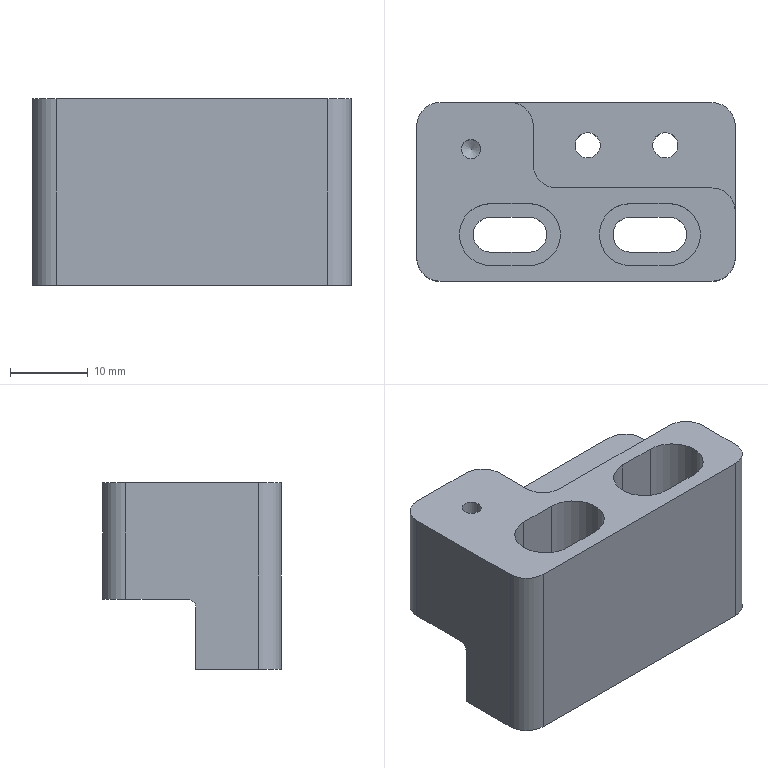Part | 1 solid | 41 faces | box 41 x 23 x 24 mm | volume 12874 mm3 | plane 21 | cylinder 19 | cone 1 | commonest cylinder face diameters 6 x7 4.5 x4 8 x4 3.242 x2 2 x1 2.459 x1
STEP:
#1=CARTESIAN_POINT('',(-14.729,5.5,-8.));
#2=VERTEX_POINT('',#1);
#3=CARTESIAN_POINT('',(-13.5,5.5,-8.));
#4=DIRECTION('',(0.,0.,1.));
#5=DIRECTION('',(-1.,0.,0.));
#6=AXIS2_PLACEMENT_3D('',#3,#4,#5);
#7=CIRCLE('',#6,1.23);
#8=EDGE_CURVE('',#2,#2,#7,.T.);
#9=ORIENTED_EDGE('',*,*,#8,.F.);
#10=EDGE_LOOP('',(#9));
#11=FACE_BOUND('',#10,.T.);
#12=CARTESIAN_POINT('',(-14.729,5.5,0.));
#13=VERTEX_POINT('',#12);
#14=CARTESIAN_POINT('',(-13.5,5.5,0.));
#15=DIRECTION('',(0.,0.,1.));
#16=DIRECTION('',(-1.,0.,0.));
#17=AXIS2_PLACEMENT_3D('',#14,#15,#16);
#18=CIRCLE('',#17,1.23);
#19=EDGE_CURVE('',#13,#13,#18,.T.);
#20=ORIENTED_EDGE('',*,*,#19,.T.);
#21=EDGE_LOOP('',(#20));
#22=FACE_BOUND('',#21,.T.);
#23=CARTESIAN_POINT('',(-13.5,5.5,0.));
#24=DIRECTION('',(0.,0.,-1.));
#25=DIRECTION('',(-1.,0.,0.));
#26=AXIS2_PLACEMENT_3D('',#23,#24,#25);
#27=CYLINDRICAL_SURFACE('',#26,1.23);
#28=ADVANCED_FACE('',(#11,#22),#27,.F.);
#29=CARTESIAN_POINT('',(-2.5,0.5,-7.5));
#30=VERTEX_POINT('',#29);
#31=CARTESIAN_POINT('',(17.5,0.5,-7.5));
#32=VERTEX_POINT('',#31);
#33=CARTESIAN_POINT('',(7.5,0.5,-7.5));
#34=DIRECTION('',(1.,0.,0.));
#35=VECTOR('',#34,1000.);
#36=LINE('',#33,#35);
#37=EDGE_CURVE('',#30,#32,#36,.T.);
#38=ORIENTED_EDGE('',*,*,#37,.F.);
#39=CARTESIAN_POINT('',(-2.5,0.5,0.));
#40=VERTEX_POINT('',#39);
#41=CARTESIAN_POINT('',(-2.5,0.5,-3.75));
#42=DIRECTION('',(0.,0.,-1.));
#43=VECTOR('',#42,1000.);
#44=LINE('',#41,#43);
#45=EDGE_CURVE('',#40,#30,#44,.T.);
#46=ORIENTED_EDGE('',*,*,#45,.F.);
#47=CARTESIAN_POINT('',(17.5,0.5,0.));
#48=VERTEX_POINT('',#47);
#49=CARTESIAN_POINT('',(7.5,0.5,0.));
#50=DIRECTION('',(1.,0.,0.));
#51=VECTOR('',#50,1000.);
#52=LINE('',#49,#51);
#53=EDGE_CURVE('',#40,#48,#52,.T.);
#54=ORIENTED_EDGE('',*,*,#53,.T.);
#55=CARTESIAN_POINT('',(17.5,0.5,-12.));
#56=DIRECTION('',(0.,0.,-1.));
#57=VECTOR('',#56,1000.);
#58=LINE('',#55,#57);
#59=EDGE_CURVE('',#48,#32,#58,.T.);
#60=ORIENTED_EDGE('',*,*,#59,.T.);
#61=EDGE_LOOP('',(#38,#46,#54,#60));
#62=FACE_BOUND('',#61,.T.);
#63=CARTESIAN_POINT('',(-5.5,0.5,0.));
#64=DIRECTION('',(0.,1.,0.));
#65=DIRECTION('',(1.,0.,0.));
#66=AXIS2_PLACEMENT_3D('',#63,#64,#65);
#67=PLANE('',#66);
#68=ADVANCED_FACE('',(#62),#67,.T.);
#69=CARTESIAN_POINT('',(-5.5,8.5,0.));
#70=VERTEX_POINT('',#69);
#71=CARTESIAN_POINT('',(-5.5,8.5,-7.5));
#72=VERTEX_POINT('',#71);
#73=CARTESIAN_POINT('',(-5.5,8.5,-7.5));
#74=DIRECTION('',(0.,0.,-1.));
#75=VECTOR('',#74,1000.);
#76=LINE('',#73,#75);
#77=EDGE_CURVE('',#70,#72,#76,.T.);
#78=ORIENTED_EDGE('',*,*,#77,.F.);
#79=CARTESIAN_POINT('',(-5.5,3.5,0.));
#80=VERTEX_POINT('',#79);
#81=CARTESIAN_POINT('',(-5.5,6.,0.));
#82=DIRECTION('',(0.,1.,0.));
#83=VECTOR('',#82,1000.);
#84=LINE('',#81,#83);
#85=EDGE_CURVE('',#80,#70,#84,.T.);
#86=ORIENTED_EDGE('',*,*,#85,.F.);
#87=CARTESIAN_POINT('',(-5.5,3.5,-7.5));
#88=VERTEX_POINT('',#87);
#89=CARTESIAN_POINT('',(-5.5,3.5,-3.75));
#90=DIRECTION('',(0.,0.,-1.));
#91=VECTOR('',#90,1000.);
#92=LINE('',#89,#91);
#93=EDGE_CURVE('',#80,#88,#92,.T.);
#94=ORIENTED_EDGE('',*,*,#93,.T.);
#95=CARTESIAN_POINT('',(-5.5,6.,-7.5));
#96=DIRECTION('',(0.,1.,0.));
#97=VECTOR('',#96,1000.);
#98=LINE('',#95,#97);
#99=EDGE_CURVE('',#88,#72,#98,.T.);
#100=ORIENTED_EDGE('',*,*,#99,.T.);
#101=EDGE_LOOP('',(#78,#86,#94,#100));
#102=FACE_BOUND('',#101,.T.);
#103=CARTESIAN_POINT('',(-5.5,0.5,0.));
#104=DIRECTION('',(-1.,0.,0.));
#105=DIRECTION('',(0.,1.,0.));
#106=AXIS2_PLACEMENT_3D('',#103,#104,#105);
#107=PLANE('',#106);
#108=ADVANCED_FACE('',(#102),#107,.F.);
#109=CARTESIAN_POINT('',(-8.5,11.5,-7.5));
#110=VERTEX_POINT('',#109);
#111=CARTESIAN_POINT('',(-8.5,8.5,-7.5));
#112=DIRECTION('',(0.,0.,1.));
#113=DIRECTION('',(-1.,0.,0.));
#114=AXIS2_PLACEMENT_3D('',#111,#112,#113);
#115=CIRCLE('',#114,3.);
#116=EDGE_CURVE('',#72,#110,#115,.T.);
#117=ORIENTED_EDGE('',*,*,#116,.T.);
#118=CARTESIAN_POINT('',(-8.5,11.5,0.));
#119=VERTEX_POINT('',#118);
#120=CARTESIAN_POINT('',(-8.5,11.5,-3.75));
#121=DIRECTION('',(0.,0.,-1.));
#122=VECTOR('',#121,1000.);
#123=LINE('',#120,#122);
#124=EDGE_CURVE('',#119,#110,#123,.T.);
#125=ORIENTED_EDGE('',*,*,#124,.F.);
#126=CARTESIAN_POINT('',(-8.5,8.5,0.));
#127=DIRECTION('',(0.,0.,1.));
#128=DIRECTION('',(-1.,0.,0.));
#129=AXIS2_PLACEMENT_3D('',#126,#127,#128);
#130=CIRCLE('',#129,3.);
#131=EDGE_CURVE('',#70,#119,#130,.T.);
#132=ORIENTED_EDGE('',*,*,#131,.F.);
#133=ORIENTED_EDGE('',*,*,#77,.T.);
#134=EDGE_LOOP('',(#117,#125,#132,#133));
#135=FACE_BOUND('',#134,.T.);
#136=CARTESIAN_POINT('',(-8.5,8.5,-7.5));
#137=DIRECTION('',(0.,0.,-1.));
#138=DIRECTION('',(0.,1.,0.));
#139=AXIS2_PLACEMENT_3D('',#136,#137,#138);
#140=CYLINDRICAL_SURFACE('',#139,3.);
#141=ADVANCED_FACE('',(#135),#140,.T.);
#142=ORIENTED_EDGE('',*,*,#124,.T.);
#143=CARTESIAN_POINT('',(17.5,11.5,-7.5));
#144=VERTEX_POINT('',#143);
#145=CARTESIAN_POINT('',(4.5,11.5,-7.5));
#146=DIRECTION('',(-1.,0.,0.));
#147=VECTOR('',#146,1000.);
#148=LINE('',#145,#147);
#149=EDGE_CURVE('',#144,#110,#148,.T.);
#150=ORIENTED_EDGE('',*,*,#149,.F.);
#151=CARTESIAN_POINT('',(17.5,11.5,-15.));
#152=VERTEX_POINT('',#151);
#153=CARTESIAN_POINT('',(17.5,11.5,-12.));
#154=DIRECTION('',(0.,0.,-1.));
#155=VECTOR('',#154,1000.);
#156=LINE('',#153,#155);
#157=EDGE_CURVE('',#144,#152,#156,.T.);
#158=ORIENTED_EDGE('',*,*,#157,.T.);
#159=CARTESIAN_POINT('',(-17.5,11.5,-15.));
#160=VERTEX_POINT('',#159);
#161=CARTESIAN_POINT('',(0.,11.5,-15.));
#162=DIRECTION('',(1.,0.,0.));
#163=VECTOR('',#162,1000.);
#164=LINE('',#161,#163);
#165=EDGE_CURVE('',#160,#152,#164,.T.);
#166=ORIENTED_EDGE('',*,*,#165,.F.);
#167=CARTESIAN_POINT('',(-17.5,11.5,0.));
#168=VERTEX_POINT('',#167);
#169=CARTESIAN_POINT('',(-17.5,11.5,-12.));
#170=DIRECTION('',(0.,0.,-1.));
#171=VECTOR('',#170,1000.);
#172=LINE('',#169,#171);
#173=EDGE_CURVE('',#168,#160,#172,.T.);
#174=ORIENTED_EDGE('',*,*,#173,.F.);
#175=CARTESIAN_POINT('',(-13.,11.5,0.));
#176=DIRECTION('',(1.,0.,0.));
#177=VECTOR('',#176,1000.);
#178=LINE('',#175,#177);
#179=EDGE_CURVE('',#168,#119,#178,.T.);
#180=ORIENTED_EDGE('',*,*,#179,.T.);
#181=EDGE_LOOP('',(#142,#150,#158,#166,#174,#180));
#182=FACE_BOUND('',#181,.T.);
#183=CARTESIAN_POINT('',(-20.5,11.5,0.));
#184=DIRECTION('',(0.,-1.,0.));
#185=DIRECTION('',(0.,0.,-1.));
#186=AXIS2_PLACEMENT_3D('',#183,#184,#185);
#187=PLANE('',#186);
#188=ADVANCED_FACE('',(#182),#187,.F.);
#189=CARTESIAN_POINT('',(-20.5,8.5,-15.));
#190=VERTEX_POINT('',#189);
#191=CARTESIAN_POINT('',(-17.5,8.5,-15.));
#192=DIRECTION('',(0.,0.,1.));
#193=DIRECTION('',(-1.,0.,0.));
#194=AXIS2_PLACEMENT_3D('',#191,#192,#193);
#195=CIRCLE('',#194,3.);
#196=EDGE_CURVE('',#160,#190,#195,.T.);
#197=ORIENTED_EDGE('',*,*,#196,.T.);
#198=CARTESIAN_POINT('',(-20.5,8.5,0.));
#199=VERTEX_POINT('',#198);
#200=CARTESIAN_POINT('',(-20.5,8.5,-7.5));
#201=DIRECTION('',(0.,0.,-1.));
#202=VECTOR('',#201,1000.);
#203=LINE('',#200,#202);
#204=EDGE_CURVE('',#199,#190,#203,.T.);
#205=ORIENTED_EDGE('',*,*,#204,.F.);
#206=CARTESIAN_POINT('',(-17.5,8.5,0.));
#207=DIRECTION('',(0.,0.,1.));
#208=DIRECTION('',(-1.,0.,0.));
#209=AXIS2_PLACEMENT_3D('',#206,#207,#208);
#210=CIRCLE('',#209,3.);
#211=EDGE_CURVE('',#168,#199,#210,.T.);
#212=ORIENTED_EDGE('',*,*,#211,.F.);
#213=ORIENTED_EDGE('',*,*,#173,.T.);
#214=EDGE_LOOP('',(#197,#205,#212,#213));
#215=FACE_BOUND('',#214,.T.);
#216=CARTESIAN_POINT('',(-17.5,8.5,-12.));
#217=DIRECTION('',(0.,0.,-1.));
#218=DIRECTION('',(-1.,0.,0.));
#219=AXIS2_PLACEMENT_3D('',#216,#217,#218);
#220=CYLINDRICAL_SURFACE('',#219,3.);
#221=ADVANCED_FACE('',(#215),#220,.T.);
#222=CARTESIAN_POINT('',(-20.5,0.5,-15.));
#223=VERTEX_POINT('',#222);
#224=CARTESIAN_POINT('',(-20.5,4.5,-15.));
#225=DIRECTION('',(0.,-1.,0.));
#226=VECTOR('',#225,1000.);
#227=LINE('',#224,#226);
#228=EDGE_CURVE('',#190,#223,#227,.T.);
#229=ORIENTED_EDGE('',*,*,#228,.T.);
#230=CARTESIAN_POINT('',(-20.5,-0.5,-16.));
#231=VERTEX_POINT('',#230);
#232=CARTESIAN_POINT('',(-20.5,0.5,-16.));
#233=DIRECTION('',(1.,0.,0.));
#234=DIRECTION('',(0.,0.,1.));
#235=AXIS2_PLACEMENT_3D('',#232,#233,#234);
#236=CIRCLE('',#235,1.);
#237=EDGE_CURVE('',#223,#231,#236,.T.);
#238=ORIENTED_EDGE('',*,*,#237,.T.);
#239=CARTESIAN_POINT('',(-20.5,-0.5,-24.));
#240=VERTEX_POINT('',#239);
#241=CARTESIAN_POINT('',(-20.5,-0.5,-20.));
#242=DIRECTION('',(0.,0.,1.));
#243=VECTOR('',#242,1000.);
#244=LINE('',#241,#243);
#245=EDGE_CURVE('',#240,#231,#244,.T.);
#246=ORIENTED_EDGE('',*,*,#245,.F.);
#247=CARTESIAN_POINT('',(-20.5,-8.5,-24.));
#248=VERTEX_POINT('',#247);
#249=CARTESIAN_POINT('',(-20.5,-4.5,-24.));
#250=DIRECTION('',(0.,1.,0.));
#251=VECTOR('',#250,1000.);
#252=LINE('',#249,#251);
#253=EDGE_CURVE('',#248,#240,#252,.T.);
#254=ORIENTED_EDGE('',*,*,#253,.F.);
#255=CARTESIAN_POINT('',(-20.5,-8.5,0.));
#256=VERTEX_POINT('',#255);
#257=CARTESIAN_POINT('',(-20.5,-8.5,-12.));
#258=DIRECTION('',(0.,0.,1.));
#259=VECTOR('',#258,1000.);
#260=LINE('',#257,#259);
#261=EDGE_CURVE('',#248,#256,#260,.T.);
#262=ORIENTED_EDGE('',*,*,#261,.T.);
#263=CARTESIAN_POINT('',(-20.5,0.,0.));
#264=DIRECTION('',(0.,-1.,0.));
#265=VECTOR('',#264,1000.);
#266=LINE('',#263,#265);
#267=EDGE_CURVE('',#199,#256,#266,.T.);
#268=ORIENTED_EDGE('',*,*,#267,.F.);
#269=ORIENTED_EDGE('',*,*,#204,.T.);
#270=EDGE_LOOP('',(#229,#238,#246,#254,#262,#268,#269));
#271=FACE_BOUND('',#270,.T.);
#272=CARTESIAN_POINT('',(-20.5,11.5,-24.));
#273=DIRECTION('',(-1.,0.,0.));
#274=DIRECTION('',(0.,-1.,0.));
#275=AXIS2_PLACEMENT_3D('',#272,#273,#274);
#276=PLANE('',#275);
#277=ADVANCED_FACE('',(#271),#276,.T.);
#278=CARTESIAN_POINT('',(-17.5,-11.5,0.));
#279=VERTEX_POINT('',#278);
#280=CARTESIAN_POINT('',(-17.5,-8.5,0.));
#281=DIRECTION('',(0.,0.,1.));
#282=DIRECTION('',(-1.,0.,0.));
#283=AXIS2_PLACEMENT_3D('',#280,#281,#282);
#284=CIRCLE('',#283,3.);
#285=EDGE_CURVE('',#256,#279,#284,.T.);
#286=ORIENTED_EDGE('',*,*,#285,.F.);
#287=ORIENTED_EDGE('',*,*,#261,.F.);
#288=CARTESIAN_POINT('',(-17.5,-11.5,-24.));
#289=VERTEX_POINT('',#288);
#290=CARTESIAN_POINT('',(-17.5,-8.5,-24.));
#291=DIRECTION('',(0.,0.,-1.));
#292=DIRECTION('',(1.,0.,0.));
#293=AXIS2_PLACEMENT_3D('',#290,#291,#292);
#294=CIRCLE('',#293,3.);
#295=EDGE_CURVE('',#289,#248,#294,.T.);
#296=ORIENTED_EDGE('',*,*,#295,.F.);
#297=CARTESIAN_POINT('',(-17.5,-11.5,-12.));
#298=DIRECTION('',(0.,0.,1.));
#299=VECTOR('',#298,1000.);
#300=LINE('',#297,#299);
#301=EDGE_CURVE('',#289,#279,#300,.T.);
#302=ORIENTED_EDGE('',*,*,#301,.T.);
#303=EDGE_LOOP('',(#286,#287,#296,#302));
#304=FACE_BOUND('',#303,.T.);
#305=CARTESIAN_POINT('',(-17.5,-8.5,-12.));
#306=DIRECTION('',(0.,0.,1.));
#307=DIRECTION('',(-1.,0.,0.));
#308=AXIS2_PLACEMENT_3D('',#305,#306,#307);
#309=CYLINDRICAL_SURFACE('',#308,3.);
#310=ADVANCED_FACE('',(#304),#309,.T.);
#311=CARTESIAN_POINT('',(17.5,-11.5,0.));
#312=VERTEX_POINT('',#311);
#313=CARTESIAN_POINT('',(20.5,-8.5,0.));
#314=VERTEX_POINT('',#313);
#315=CARTESIAN_POINT('',(17.5,-8.5,0.));
#316=DIRECTION('',(0.,0.,1.));
#317=DIRECTION('',(-1.,0.,0.));
#318=AXIS2_PLACEMENT_3D('',#315,#316,#317);
#319=CIRCLE('',#318,3.);
#320=EDGE_CURVE('',#312,#314,#319,.T.);
#321=ORIENTED_EDGE('',*,*,#320,.F.);
#322=CARTESIAN_POINT('',(17.5,-11.5,-24.));
#323=VERTEX_POINT('',#322);
#324=CARTESIAN_POINT('',(17.5,-11.5,-12.));
#325=DIRECTION('',(0.,0.,1.));
#326=VECTOR('',#325,1000.);
#327=LINE('',#324,#326);
#328=EDGE_CURVE('',#323,#312,#327,.T.);
#329=ORIENTED_EDGE('',*,*,#328,.F.);
#330=CARTESIAN_POINT('',(20.5,-8.5,-24.));
#331=VERTEX_POINT('',#330);
#332=CARTESIAN_POINT('',(17.5,-8.5,-24.));
#333=DIRECTION('',(0.,0.,-1.));
#334=DIRECTION('',(1.,0.,0.));
#335=AXIS2_PLACEMENT_3D('',#332,#333,#334);
#336=CIRCLE('',#335,3.);
#337=EDGE_CURVE('',#331,#323,#336,.T.);
#338=ORIENTED_EDGE('',*,*,#337,.F.);
#339=CARTESIAN_POINT('',(20.5,-8.5,-12.));
#340=DIRECTION('',(0.,0.,1.));
#341=VECTOR('',#340,1000.);
#342=LINE('',#339,#341);
#343=EDGE_CURVE('',#331,#314,#342,.T.);
#344=ORIENTED_EDGE('',*,*,#343,.T.);
#345=EDGE_LOOP('',(#321,#329,#338,#344));
#346=FACE_BOUND('',#345,.T.);
#347=CARTESIAN_POINT('',(17.5,-8.5,-12.));
#348=DIRECTION('',(0.,0.,1.));
#349=DIRECTION('',(0.,-1.,0.));
#350=AXIS2_PLACEMENT_3D('',#347,#348,#349);
#351=CYLINDRICAL_SURFACE('',#350,3.);
#352=ADVANCED_FACE('',(#346),#351,.T.);
#353=CARTESIAN_POINT('',(20.5,-2.5,-7.5));
#354=VERTEX_POINT('',#353);
#355=CARTESIAN_POINT('',(17.5,-2.5,-7.5));
#356=DIRECTION('',(0.,0.,1.));
#357=DIRECTION('',(-1.,0.,0.));
#358=AXIS2_PLACEMENT_3D('',#355,#356,#357);
#359=CIRCLE('',#358,3.);
#360=EDGE_CURVE('',#354,#32,#359,.T.);
#361=ORIENTED_EDGE('',*,*,#360,.T.);
#362=ORIENTED_EDGE('',*,*,#59,.F.);
#363=CARTESIAN_POINT('',(20.5,-2.5,0.));
#364=VERTEX_POINT('',#363);
#365=CARTESIAN_POINT('',(17.5,-2.5,0.));
#366=DIRECTION('',(0.,0.,1.));
#367=DIRECTION('',(-1.,0.,0.));
#368=AXIS2_PLACEMENT_3D('',#365,#366,#367);
#369=CIRCLE('',#368,3.);
#370=EDGE_CURVE('',#364,#48,#369,.T.);
#371=ORIENTED_EDGE('',*,*,#370,.F.);
#372=CARTESIAN_POINT('',(20.5,-2.5,-3.75));
#373=DIRECTION('',(0.,0.,-1.));
#374=VECTOR('',#373,1000.);
#375=LINE('',#372,#374);
#376=EDGE_CURVE('',#364,#354,#375,.T.);
#377=ORIENTED_EDGE('',*,*,#376,.T.);
#378=EDGE_LOOP('',(#361,#362,#371,#377));
#379=FACE_BOUND('',#378,.T.);
#380=CARTESIAN_POINT('',(17.5,-2.5,-12.));
#381=DIRECTION('',(0.,0.,-1.));
#382=DIRECTION('',(0.,1.,0.));
#383=AXIS2_PLACEMENT_3D('',#380,#381,#382);
#384=CYLINDRICAL_SURFACE('',#383,3.);
#385=ADVANCED_FACE('',(#379),#384,.T.);
#386=CARTESIAN_POINT('',(7.,-9.5,-10.));
#387=VERTEX_POINT('',#386);
#388=CARTESIAN_POINT('',(7.,-1.5,-10.));
#389=VERTEX_POINT('',#388);
#390=CARTESIAN_POINT('',(7.,-5.5,-10.));
#391=DIRECTION('',(0.,0.,-1.));
#392=DIRECTION('',(1.,0.,0.));
#393=AXIS2_PLACEMENT_3D('',#390,#391,#392);
#394=CIRCLE('',#393,4.);
#395=EDGE_CURVE('',#387,#389,#394,.T.);
#396=ORIENTED_EDGE('',*,*,#395,.T.);
#397=CARTESIAN_POINT('',(7.,-1.5,0.));
#398=VERTEX_POINT('',#397);
#399=CARTESIAN_POINT('',(7.,-1.5,-5.));
#400=DIRECTION('',(0.,0.,-1.));
#401=VECTOR('',#400,1000.);
#402=LINE('',#399,#401);
#403=EDGE_CURVE('',#398,#389,#402,.T.);
#404=ORIENTED_EDGE('',*,*,#403,.F.);
#405=CARTESIAN_POINT('',(7.,-9.5,0.));
#406=VERTEX_POINT('',#405);
#407=CARTESIAN_POINT('',(7.,-5.5,0.));
#408=DIRECTION('',(0.,0.,1.));
#409=DIRECTION('',(-1.,0.,0.));
#410=AXIS2_PLACEMENT_3D('',#407,#408,#409);
#411=CIRCLE('',#410,4.);
#412=EDGE_CURVE('',#398,#406,#411,.T.);
#413=ORIENTED_EDGE('',*,*,#412,.T.);
#414=CARTESIAN_POINT('',(7.,-9.5,-5.));
#415=DIRECTION('',(0.,0.,-1.));
#416=VECTOR('',#415,1000.);
#417=LINE('',#414,#416);
#418=EDGE_CURVE('',#406,#387,#417,.T.);
#419=ORIENTED_EDGE('',*,*,#418,.T.);
#420=EDGE_LOOP('',(#396,#404,#413,#419));
#421=FACE_BOUND('',#420,.T.);
#422=CARTESIAN_POINT('',(7.,-5.5,-5.61));
#423=DIRECTION('',(0.,0.,1.));
#424=DIRECTION('',(0.,1.,0.));
#425=AXIS2_PLACEMENT_3D('',#422,#423,#424);
#426=CYLINDRICAL_SURFACE('',#425,4.);
#427=ADVANCED_FACE('',(#421),#426,.F.);
#428=CARTESIAN_POINT('',(12.,-1.5,0.));
#429=VERTEX_POINT('',#428);
#430=CARTESIAN_POINT('',(9.5,-1.5,0.));
#431=DIRECTION('',(1.,0.,0.));
#432=VECTOR('',#431,1000.);
#433=LINE('',#430,#432);
#434=EDGE_CURVE('',#398,#429,#433,.T.);
#435=ORIENTED_EDGE('',*,*,#434,.F.);
#436=ORIENTED_EDGE('',*,*,#403,.T.);
#437=CARTESIAN_POINT('',(12.,-1.5,-10.));
#438=VERTEX_POINT('',#437);
#439=CARTESIAN_POINT('',(9.5,-1.5,-10.));
#440=DIRECTION('',(1.,0.,0.));
#441=VECTOR('',#440,1000.);
#442=LINE('',#439,#441);
#443=EDGE_CURVE('',#389,#438,#442,.T.);
#444=ORIENTED_EDGE('',*,*,#443,.T.);
#445=CARTESIAN_POINT('',(12.,-1.5,-5.61));
#446=DIRECTION('',(0.,0.,1.));
#447=VECTOR('',#446,1000.);
#448=LINE('',#445,#447);
#449=EDGE_CURVE('',#438,#429,#448,.T.);
#450=ORIENTED_EDGE('',*,*,#449,.T.);
#451=EDGE_LOOP('',(#435,#436,#444,#450));
#452=FACE_BOUND('',#451,.T.);
#453=CARTESIAN_POINT('',(-11.,-1.5,0.));
#454=DIRECTION('',(0.,1.,0.));
#455=DIRECTION('',(1.,0.,0.));
#456=AXIS2_PLACEMENT_3D('',#453,#454,#455);
#457=PLANE('',#456);
#458=ADVANCED_FACE('',(#452),#457,.F.);
#459=CARTESIAN_POINT('',(12.,-9.5,-10.));
#460=VERTEX_POINT('',#459);
#461=CARTESIAN_POINT('',(12.,-5.5,-10.));
#462=DIRECTION('',(0.,0.,-1.));
#463=DIRECTION('',(1.,0.,0.));
#464=AXIS2_PLACEMENT_3D('',#461,#462,#463);
#465=CIRCLE('',#464,4.);
#466=EDGE_CURVE('',#438,#460,#465,.T.);
#467=ORIENTED_EDGE('',*,*,#466,.T.);
#468=CARTESIAN_POINT('',(12.,-9.5,0.));
#469=VERTEX_POINT('',#468);
#470=CARTESIAN_POINT('',(12.,-9.5,-5.));
#471=DIRECTION('',(0.,0.,-1.));
#472=VECTOR('',#471,1000.);
#473=LINE('',#470,#472);
#474=EDGE_CURVE('',#469,#460,#473,.T.);
#475=ORIENTED_EDGE('',*,*,#474,.F.);
#476=CARTESIAN_POINT('',(12.,-5.5,0.));
#477=DIRECTION('',(0.,0.,1.));
#478=DIRECTION('',(-1.,0.,0.));
#479=AXIS2_PLACEMENT_3D('',#476,#477,#478);
#480=CIRCLE('',#479,4.);
#481=EDGE_CURVE('',#469,#429,#480,.T.);
#482=ORIENTED_EDGE('',*,*,#481,.T.);
#483=ORIENTED_EDGE('',*,*,#449,.F.);
#484=EDGE_LOOP('',(#467,#475,#482,#483));
#485=FACE_BOUND('',#484,.T.);
#486=CARTESIAN_POINT('',(12.,-5.5,-5.61));
#487=DIRECTION('',(0.,0.,1.));
#488=DIRECTION('',(0.,-1.,0.));
#489=AXIS2_PLACEMENT_3D('',#486,#487,#488);
#490=CYLINDRICAL_SURFACE('',#489,4.);
#491=ADVANCED_FACE('',(#485),#490,.F.);
#492=CARTESIAN_POINT('',(9.5,-9.5,0.));
#493=DIRECTION('',(-1.,0.,0.));
#494=VECTOR('',#493,1000.);
#495=LINE('',#492,#494);
#496=EDGE_CURVE('',#469,#406,#495,.T.);
#497=ORIENTED_EDGE('',*,*,#496,.F.);
#498=ORIENTED_EDGE('',*,*,#474,.T.);
#499=CARTESIAN_POINT('',(9.5,-9.5,-10.));
#500=DIRECTION('',(-1.,0.,0.));
#501=VECTOR('',#500,1000.);
#502=LINE('',#499,#501);
#503=EDGE_CURVE('',#460,#387,#502,.T.);
#504=ORIENTED_EDGE('',*,*,#503,.T.);
#505=ORIENTED_EDGE('',*,*,#418,.F.);
#506=EDGE_LOOP('',(#497,#498,#504,#505));
#507=FACE_BOUND('',#506,.T.);
#508=CARTESIAN_POINT('',(-6.,-9.5,0.));
#509=DIRECTION('',(0.,-1.,0.));
#510=DIRECTION('',(-1.,0.,0.));
#511=AXIS2_PLACEMENT_3D('',#508,#509,#510);
#512=PLANE('',#511);
#513=ADVANCED_FACE('',(#507),#512,.F.);
#514=CARTESIAN_POINT('',(-11.,-9.5,-10.));
#515=VERTEX_POINT('',#514);
#516=CARTESIAN_POINT('',(-11.,-1.5,-10.));
#517=VERTEX_POINT('',#516);
#518=CARTESIAN_POINT('',(-11.,-5.5,-10.));
#519=DIRECTION('',(0.,0.,-1.));
#520=DIRECTION('',(1.,0.,0.));
#521=AXIS2_PLACEMENT_3D('',#518,#519,#520);
#522=CIRCLE('',#521,4.);
#523=EDGE_CURVE('',#515,#517,#522,.T.);
#524=ORIENTED_EDGE('',*,*,#523,.T.);
#525=CARTESIAN_POINT('',(-11.,-1.5,0.));
#526=VERTEX_POINT('',#525);
#527=CARTESIAN_POINT('',(-11.,-1.5,-5.));
#528=DIRECTION('',(0.,0.,-1.));
#529=VECTOR('',#528,1000.);
#530=LINE('',#527,#529);
#531=EDGE_CURVE('',#526,#517,#530,.T.);
#532=ORIENTED_EDGE('',*,*,#531,.F.);
#533=CARTESIAN_POINT('',(-11.,-9.5,0.));
#534=VERTEX_POINT('',#533);
#535=CARTESIAN_POINT('',(-11.,-5.5,0.));
#536=DIRECTION('',(0.,0.,1.));
#537=DIRECTION('',(-1.,0.,0.));
#538=AXIS2_PLACEMENT_3D('',#535,#536,#537);
#539=CIRCLE('',#538,4.);
#540=EDGE_CURVE('',#526,#534,#539,.T.);
#541=ORIENTED_EDGE('',*,*,#540,.T.);
#542=CARTESIAN_POINT('',(-11.,-9.5,-5.));
#543=DIRECTION('',(0.,0.,-1.));
#544=VECTOR('',#543,1000.);
#545=LINE('',#542,#544);
#546=EDGE_CURVE('',#534,#515,#545,.T.);
#547=ORIENTED_EDGE('',*,*,#546,.T.);
#548=EDGE_LOOP('',(#524,#532,#541,#547));
#549=FACE_BOUND('',#548,.T.);
#550=CARTESIAN_POINT('',(-11.,-5.5,-5.61));
#551=DIRECTION('',(0.,0.,1.));
#552=DIRECTION('',(0.,1.,0.));
#553=AXIS2_PLACEMENT_3D('',#550,#551,#552);
#554=CYLINDRICAL_SURFACE('',#553,4.);
#555=ADVANCED_FACE('',(#549),#554,.F.);
#556=CARTESIAN_POINT('',(-6.,-1.5,0.));
#557=VERTEX_POINT('',#556);
#558=CARTESIAN_POINT('',(-8.5,-1.5,0.));
#559=DIRECTION('',(1.,0.,0.));
#560=VECTOR('',#559,1000.);
#561=LINE('',#558,#560);
#562=EDGE_CURVE('',#526,#557,#561,.T.);
#563=ORIENTED_EDGE('',*,*,#562,.F.);
#564=ORIENTED_EDGE('',*,*,#531,.T.);
#565=CARTESIAN_POINT('',(-6.,-1.5,-10.));
#566=VERTEX_POINT('',#565);
#567=CARTESIAN_POINT('',(-8.5,-1.5,-10.));
#568=DIRECTION('',(1.,0.,0.));
#569=VECTOR('',#568,1000.);
#570=LINE('',#567,#569);
#571=EDGE_CURVE('',#517,#566,#570,.T.);
#572=ORIENTED_EDGE('',*,*,#571,.T.);
#573=CARTESIAN_POINT('',(-6.,-1.5,-5.61));
#574=DIRECTION('',(0.,0.,1.));
#575=VECTOR('',#574,1000.);
#576=LINE('',#573,#575);
#577=EDGE_CURVE('',#566,#557,#576,.T.);
#578=ORIENTED_EDGE('',*,*,#577,.T.);
#579=EDGE_LOOP('',(#563,#564,#572,#578));
#580=FACE_BOUND('',#579,.T.);
#581=CARTESIAN_POINT('',(-11.,-1.5,0.));
#582=DIRECTION('',(0.,1.,0.));
#583=DIRECTION('',(1.,0.,0.));
#584=AXIS2_PLACEMENT_3D('',#581,#582,#583);
#585=PLANE('',#584);
#586=ADVANCED_FACE('',(#580),#585,.F.);
#587=CARTESIAN_POINT('',(-6.,-9.5,-10.));
#588=VERTEX_POINT('',#587);
#589=CARTESIAN_POINT('',(-6.,-5.5,-10.));
#590=DIRECTION('',(0.,0.,-1.));
#591=DIRECTION('',(1.,0.,0.));
#592=AXIS2_PLACEMENT_3D('',#589,#590,#591);
#593=CIRCLE('',#592,4.);
#594=EDGE_CURVE('',#566,#588,#593,.T.);
#595=ORIENTED_EDGE('',*,*,#594,.T.);
#596=CARTESIAN_POINT('',(-6.,-9.5,0.));
#597=VERTEX_POINT('',#596);
#598=CARTESIAN_POINT('',(-6.,-9.5,-5.));
#599=DIRECTION('',(0.,0.,-1.));
#600=VECTOR('',#599,1000.);
#601=LINE('',#598,#600);
#602=EDGE_CURVE('',#597,#588,#601,.T.);
#603=ORIENTED_EDGE('',*,*,#602,.F.);
#604=CARTESIAN_POINT('',(-6.,-5.5,0.));
#605=DIRECTION('',(0.,0.,1.));
#606=DIRECTION('',(-1.,0.,0.));
#607=AXIS2_PLACEMENT_3D('',#604,#605,#606);
#608=CIRCLE('',#607,4.);
#609=EDGE_CURVE('',#597,#557,#608,.T.);
#610=ORIENTED_EDGE('',*,*,#609,.T.);
#611=ORIENTED_EDGE('',*,*,#577,.F.);
#612=EDGE_LOOP('',(#595,#603,#610,#611));
#613=FACE_BOUND('',#612,.T.);
#614=CARTESIAN_POINT('',(-6.,-5.5,-5.61));
#615=DIRECTION('',(0.,0.,1.));
#616=DIRECTION('',(0.,-1.,0.));
#617=AXIS2_PLACEMENT_3D('',#614,#615,#616);
#618=CYLINDRICAL_SURFACE('',#617,4.);
#619=ADVANCED_FACE('',(#613),#618,.F.);
#620=CARTESIAN_POINT('',(-8.5,-9.5,0.));
#621=DIRECTION('',(-1.,0.,0.));
#622=VECTOR('',#621,1000.);
#623=LINE('',#620,#622);
#624=EDGE_CURVE('',#597,#534,#623,.T.);
#625=ORIENTED_EDGE('',*,*,#624,.F.);
#626=ORIENTED_EDGE('',*,*,#602,.T.);
#627=CARTESIAN_POINT('',(-8.5,-9.5,-10.));
#628=DIRECTION('',(-1.,0.,0.));
#629=VECTOR('',#628,1000.);
#630=LINE('',#627,#629);
#631=EDGE_CURVE('',#588,#515,#630,.T.);
#632=ORIENTED_EDGE('',*,*,#631,.T.);
#633=ORIENTED_EDGE('',*,*,#546,.F.);
#634=EDGE_LOOP('',(#625,#626,#632,#633));
#635=FACE_BOUND('',#634,.T.);
#636=CARTESIAN_POINT('',(-6.,-9.5,0.));
#637=DIRECTION('',(0.,-1.,0.));
#638=DIRECTION('',(-1.,0.,0.));
#639=AXIS2_PLACEMENT_3D('',#636,#637,#638);
#640=PLANE('',#639);
#641=ADVANCED_FACE('',(#635),#640,.F.);
#642=CARTESIAN_POINT('',(13.121,6.,-7.5));
#643=VERTEX_POINT('',#642);
#644=CARTESIAN_POINT('',(11.5,6.,-7.5));
#645=DIRECTION('',(0.,0.,-1.));
#646=DIRECTION('',(1.,0.,0.));
#647=AXIS2_PLACEMENT_3D('',#644,#645,#646);
#648=CIRCLE('',#647,1.621);
#649=EDGE_CURVE('',#643,#643,#648,.T.);
#650=ORIENTED_EDGE('',*,*,#649,.T.);
#651=EDGE_LOOP('',(#650));
#652=FACE_BOUND('',#651,.T.);
#653=CARTESIAN_POINT('',(3.121,6.,-7.5));
#654=VERTEX_POINT('',#653);
#655=CARTESIAN_POINT('',(1.5,6.,-7.5));
#656=DIRECTION('',(0.,0.,-1.));
#657=DIRECTION('',(1.,0.,0.));
#658=AXIS2_PLACEMENT_3D('',#655,#656,#657);
#659=CIRCLE('',#658,1.621);
#660=EDGE_CURVE('',#654,#654,#659,.T.);
#661=ORIENTED_EDGE('',*,*,#660,.T.);
#662=EDGE_LOOP('',(#661));
#663=FACE_BOUND('',#662,.T.);
#664=ORIENTED_EDGE('',*,*,#360,.F.);
#665=CARTESIAN_POINT('',(20.5,8.5,-7.5));
#666=VERTEX_POINT('',#665);
#667=CARTESIAN_POINT('',(20.5,3.,-7.5));
#668=DIRECTION('',(0.,-1.,0.));
#669=VECTOR('',#668,1000.);
#670=LINE('',#667,#669);
#671=EDGE_CURVE('',#666,#354,#670,.T.);
#672=ORIENTED_EDGE('',*,*,#671,.F.);
#673=CARTESIAN_POINT('',(17.5,8.5,-7.5));
#674=DIRECTION('',(0.,0.,-1.));
#675=DIRECTION('',(1.,0.,0.));
#676=AXIS2_PLACEMENT_3D('',#673,#674,#675);
#677=CIRCLE('',#676,3.);
#678=EDGE_CURVE('',#144,#666,#677,.T.);
#679=ORIENTED_EDGE('',*,*,#678,.F.);
#680=ORIENTED_EDGE('',*,*,#149,.T.);
#681=ORIENTED_EDGE('',*,*,#116,.F.);
#682=ORIENTED_EDGE('',*,*,#99,.F.);
#683=CARTESIAN_POINT('',(-2.5,3.5,-7.5));
#684=DIRECTION('',(0.,0.,-1.));
#685=DIRECTION('',(1.,0.,0.));
#686=AXIS2_PLACEMENT_3D('',#683,#684,#685);
#687=CIRCLE('',#686,3.);
#688=EDGE_CURVE('',#30,#88,#687,.T.);
#689=ORIENTED_EDGE('',*,*,#688,.F.);
#690=ORIENTED_EDGE('',*,*,#37,.T.);
#691=EDGE_LOOP('',(#664,#672,#679,#680,#681,#682,#689,#690));
#692=FACE_BOUND('',#691,.T.);
#693=CARTESIAN_POINT('',(-20.5,11.5,-7.5));
#694=DIRECTION('',(0.,0.,1.));
#695=DIRECTION('',(-1.,0.,0.));
#696=AXIS2_PLACEMENT_3D('',#693,#694,#695);
#697=PLANE('',#696);
#698=ADVANCED_FACE('',(#652,#663,#692),#697,.T.);
#699=CARTESIAN_POINT('',(20.5,8.5,-15.));
#700=VERTEX_POINT('',#699);
#701=CARTESIAN_POINT('',(20.5,8.5,-11.25));
#702=DIRECTION('',(0.,0.,-1.));
#703=VECTOR('',#702,1000.);
#704=LINE('',#701,#703);
#705=EDGE_CURVE('',#666,#700,#704,.T.);
#706=ORIENTED_EDGE('',*,*,#705,.T.);
#707=CARTESIAN_POINT('',(17.5,8.5,-15.));
#708=DIRECTION('',(0.,0.,1.));
#709=DIRECTION('',(-1.,0.,0.));
#710=AXIS2_PLACEMENT_3D('',#707,#708,#709);
#711=CIRCLE('',#710,3.);
#712=EDGE_CURVE('',#700,#152,#711,.T.);
#713=ORIENTED_EDGE('',*,*,#712,.T.);
#714=ORIENTED_EDGE('',*,*,#157,.F.);
#715=ORIENTED_EDGE('',*,*,#678,.T.);
#716=EDGE_LOOP('',(#706,#713,#714,#715));
#717=FACE_BOUND('',#716,.T.);
#718=CARTESIAN_POINT('',(17.5,8.5,-12.));
#719=DIRECTION('',(0.,0.,-1.));
#720=DIRECTION('',(0.,1.,0.));
#721=AXIS2_PLACEMENT_3D('',#718,#719,#720);
#722=CYLINDRICAL_SURFACE('',#721,3.);
#723=ADVANCED_FACE('',(#717),#722,.T.);
#724=CARTESIAN_POINT('',(13.121,6.,-15.));
#725=VERTEX_POINT('',#724);
#726=CARTESIAN_POINT('',(11.5,6.,-15.));
#727=DIRECTION('',(0.,0.,-1.));
#728=DIRECTION('',(1.,0.,0.));
#729=AXIS2_PLACEMENT_3D('',#726,#727,#728);
#730=CIRCLE('',#729,1.621);
#731=EDGE_CURVE('',#725,#725,#730,.T.);
#732=ORIENTED_EDGE('',*,*,#731,.F.);
#733=EDGE_LOOP('',(#732));
#734=FACE_BOUND('',#733,.T.);
#735=CARTESIAN_POINT('',(3.121,6.,-15.));
#736=VERTEX_POINT('',#735);
#737=CARTESIAN_POINT('',(1.5,6.,-15.));
#738=DIRECTION('',(0.,0.,-1.));
#739=DIRECTION('',(1.,0.,0.));
#740=AXIS2_PLACEMENT_3D('',#737,#738,#739);
#741=CIRCLE('',#740,1.621);
#742=EDGE_CURVE('',#736,#736,#741,.T.);
#743=ORIENTED_EDGE('',*,*,#742,.F.);
#744=EDGE_LOOP('',(#743));
#745=FACE_BOUND('',#744,.T.);
#746=ORIENTED_EDGE('',*,*,#712,.F.);
#747=CARTESIAN_POINT('',(20.5,0.5,-15.));
#748=VERTEX_POINT('',#747);
#749=CARTESIAN_POINT('',(20.5,4.5,-15.));
#750=DIRECTION('',(0.,-1.,0.));
#751=VECTOR('',#750,1000.);
#752=LINE('',#749,#751);
#753=EDGE_CURVE('',#700,#748,#752,.T.);
#754=ORIENTED_EDGE('',*,*,#753,.T.);
#755=CARTESIAN_POINT('',(0.,0.5,-15.));
#756=DIRECTION('',(1.,0.,0.));
#757=VECTOR('',#756,1000.);
#758=LINE('',#755,#757);
#759=EDGE_CURVE('',#223,#748,#758,.T.);
#760=ORIENTED_EDGE('',*,*,#759,.F.);
#761=ORIENTED_EDGE('',*,*,#228,.F.);
#762=ORIENTED_EDGE('',*,*,#196,.F.);
#763=ORIENTED_EDGE('',*,*,#165,.T.);
#764=EDGE_LOOP('',(#746,#754,#760,#761,#762,#763));
#765=FACE_BOUND('',#764,.T.);
#766=CARTESIAN_POINT('',(-20.5,11.5,-15.));
#767=DIRECTION('',(0.,0.,1.));
#768=DIRECTION('',(0.,-1.,0.));
#769=AXIS2_PLACEMENT_3D('',#766,#767,#768);
#770=PLANE('',#769);
#771=ADVANCED_FACE('',(#734,#745,#765),#770,.F.);
#772=CARTESIAN_POINT('',(20.5,-0.5,-24.));
#773=VERTEX_POINT('',#772);
#774=CARTESIAN_POINT('',(20.5,-0.5,-16.));
#775=VERTEX_POINT('',#774);
#776=CARTESIAN_POINT('',(20.5,-0.5,-20.));
#777=DIRECTION('',(0.,0.,1.));
#778=VECTOR('',#777,1000.);
#779=LINE('',#776,#778);
#780=EDGE_CURVE('',#773,#775,#779,.T.);
#781=ORIENTED_EDGE('',*,*,#780,.F.);
#782=CARTESIAN_POINT('',(0.,-0.5,-24.));
#783=DIRECTION('',(1.,0.,0.));
#784=VECTOR('',#783,1000.);
#785=LINE('',#782,#784);
#786=EDGE_CURVE('',#240,#773,#785,.T.);
#787=ORIENTED_EDGE('',*,*,#786,.F.);
#788=ORIENTED_EDGE('',*,*,#245,.T.);
#789=CARTESIAN_POINT('',(0.,-0.5,-16.));
#790=DIRECTION('',(1.,0.,0.));
#791=VECTOR('',#790,1000.);
#792=LINE('',#789,#791);
#793=EDGE_CURVE('',#231,#775,#792,.T.);
#794=ORIENTED_EDGE('',*,*,#793,.T.);
#795=EDGE_LOOP('',(#781,#787,#788,#794));
#796=FACE_BOUND('',#795,.T.);
#797=CARTESIAN_POINT('',(-20.5,-0.5,-24.));
#798=DIRECTION('',(0.,1.,0.));
#799=DIRECTION('',(0.,0.,1.));
#800=AXIS2_PLACEMENT_3D('',#797,#798,#799);
#801=PLANE('',#800);
#802=ADVANCED_FACE('',(#796),#801,.T.);
#803=CARTESIAN_POINT('',(12.,-3.25,-10.));
#804=VERTEX_POINT('',#803);
#805=CARTESIAN_POINT('',(12.,-7.75,-10.));
#806=VERTEX_POINT('',#805);
#807=CARTESIAN_POINT('',(12.,-5.5,-10.));
#808=DIRECTION('',(0.,0.,-1.));
#809=DIRECTION('',(1.,0.,0.));
#810=AXIS2_PLACEMENT_3D('',#807,#808,#809);
#811=CIRCLE('',#810,2.25);
#812=EDGE_CURVE('',#804,#806,#811,.T.);
#813=ORIENTED_EDGE('',*,*,#812,.F.);
#814=CARTESIAN_POINT('',(12.,-3.25,-24.));
#815=VERTEX_POINT('',#814);
#816=CARTESIAN_POINT('',(12.,-3.25,-17.));
#817=DIRECTION('',(0.,0.,-1.));
#818=VECTOR('',#817,1000.);
#819=LINE('',#816,#818);
#820=EDGE_CURVE('',#804,#815,#819,.T.);
#821=ORIENTED_EDGE('',*,*,#820,.T.);
#822=CARTESIAN_POINT('',(12.,-7.75,-24.));
#823=VERTEX_POINT('',#822);
#824=CARTESIAN_POINT('',(12.,-5.5,-24.));
#825=DIRECTION('',(0.,0.,-1.));
#826=DIRECTION('',(1.,0.,0.));
#827=AXIS2_PLACEMENT_3D('',#824,#825,#826);
#828=CIRCLE('',#827,2.25);
#829=EDGE_CURVE('',#815,#823,#828,.T.);
#830=ORIENTED_EDGE('',*,*,#829,.T.);
#831=CARTESIAN_POINT('',(12.,-7.75,-17.));
#832=DIRECTION('',(0.,0.,-1.));
#833=VECTOR('',#832,1000.);
#834=LINE('',#831,#833);
#835=EDGE_CURVE('',#806,#823,#834,.T.);
#836=ORIENTED_EDGE('',*,*,#835,.F.);
#837=EDGE_LOOP('',(#813,#821,#830,#836));
#838=FACE_BOUND('',#837,.T.);
#839=CARTESIAN_POINT('',(12.,-5.5,-12.66));
#840=DIRECTION('',(0.,0.,1.));
#841=DIRECTION('',(0.,-1.,0.));
#842=AXIS2_PLACEMENT_3D('',#839,#840,#841);
#843=CYLINDRICAL_SURFACE('',#842,2.25);
#844=ADVANCED_FACE('',(#838),#843,.F.);
#845=CARTESIAN_POINT('',(7.,-3.25,-10.));
#846=VERTEX_POINT('',#845);
#847=CARTESIAN_POINT('',(9.5,-3.25,-10.));
#848=DIRECTION('',(1.,0.,0.));
#849=VECTOR('',#848,1000.);
#850=LINE('',#847,#849);
#851=EDGE_CURVE('',#846,#804,#850,.T.);
#852=ORIENTED_EDGE('',*,*,#851,.F.);
#853=CARTESIAN_POINT('',(7.,-3.25,-24.));
#854=VERTEX_POINT('',#853);
#855=CARTESIAN_POINT('',(7.,-3.25,-12.66));
#856=DIRECTION('',(0.,0.,1.));
#857=VECTOR('',#856,1000.);
#858=LINE('',#855,#857);
#859=EDGE_CURVE('',#854,#846,#858,.T.);
#860=ORIENTED_EDGE('',*,*,#859,.F.);
#861=CARTESIAN_POINT('',(9.5,-3.25,-24.));
#862=DIRECTION('',(1.,0.,0.));
#863=VECTOR('',#862,1000.);
#864=LINE('',#861,#863);
#865=EDGE_CURVE('',#854,#815,#864,.T.);
#866=ORIENTED_EDGE('',*,*,#865,.T.);
#867=ORIENTED_EDGE('',*,*,#820,.F.);
#868=EDGE_LOOP('',(#852,#860,#866,#867));
#869=FACE_BOUND('',#868,.T.);
#870=CARTESIAN_POINT('',(-11.,-3.25,0.));
#871=DIRECTION('',(0.,1.,0.));
#872=DIRECTION('',(1.,0.,0.));
#873=AXIS2_PLACEMENT_3D('',#870,#871,#872);
#874=PLANE('',#873);
#875=ADVANCED_FACE('',(#869),#874,.F.);
#876=ORIENTED_EDGE('',*,*,#859,.T.);
#877=CARTESIAN_POINT('',(7.,-7.75,-10.));
#878=VERTEX_POINT('',#877);
#879=CARTESIAN_POINT('',(7.,-5.5,-10.));
#880=DIRECTION('',(0.,0.,-1.));
#881=DIRECTION('',(1.,0.,0.));
#882=AXIS2_PLACEMENT_3D('',#879,#880,#881);
#883=CIRCLE('',#882,2.25);
#884=EDGE_CURVE('',#878,#846,#883,.T.);
#885=ORIENTED_EDGE('',*,*,#884,.F.);
#886=CARTESIAN_POINT('',(7.,-7.75,-24.));
#887=VERTEX_POINT('',#886);
#888=CARTESIAN_POINT('',(7.,-7.75,-17.));
#889=DIRECTION('',(0.,0.,-1.));
#890=VECTOR('',#889,1000.);
#891=LINE('',#888,#890);
#892=EDGE_CURVE('',#878,#887,#891,.T.);
#893=ORIENTED_EDGE('',*,*,#892,.T.);
#894=CARTESIAN_POINT('',(7.,-5.5,-24.));
#895=DIRECTION('',(0.,0.,-1.));
#896=DIRECTION('',(1.,0.,0.));
#897=AXIS2_PLACEMENT_3D('',#894,#895,#896);
#898=CIRCLE('',#897,2.25);
#899=EDGE_CURVE('',#887,#854,#898,.T.);
#900=ORIENTED_EDGE('',*,*,#899,.T.);
#901=EDGE_LOOP('',(#876,#885,#893,#900));
#902=FACE_BOUND('',#901,.T.);
#903=CARTESIAN_POINT('',(7.,-5.5,-12.66));
#904=DIRECTION('',(0.,0.,1.));
#905=DIRECTION('',(0.,1.,0.));
#906=AXIS2_PLACEMENT_3D('',#903,#904,#905);
#907=CYLINDRICAL_SURFACE('',#906,2.25);
#908=ADVANCED_FACE('',(#902),#907,.F.);
#909=CARTESIAN_POINT('',(9.5,-7.75,-10.));
#910=DIRECTION('',(-1.,0.,0.));
#911=VECTOR('',#910,1000.);
#912=LINE('',#909,#911);
#913=EDGE_CURVE('',#806,#878,#912,.T.);
#914=ORIENTED_EDGE('',*,*,#913,.F.);
#915=ORIENTED_EDGE('',*,*,#835,.T.);
#916=CARTESIAN_POINT('',(9.5,-7.75,-24.));
#917=DIRECTION('',(-1.,0.,0.));
#918=VECTOR('',#917,1000.);
#919=LINE('',#916,#918);
#920=EDGE_CURVE('',#823,#887,#919,.T.);
#921=ORIENTED_EDGE('',*,*,#920,.T.);
#922=ORIENTED_EDGE('',*,*,#892,.F.);
#923=EDGE_LOOP('',(#914,#915,#921,#922));
#924=FACE_BOUND('',#923,.T.);
#925=CARTESIAN_POINT('',(-6.,-7.75,0.));
#926=DIRECTION('',(0.,-1.,0.));
#927=DIRECTION('',(-1.,0.,0.));
#928=AXIS2_PLACEMENT_3D('',#925,#926,#927);
#929=PLANE('',#928);
#930=ADVANCED_FACE('',(#924),#929,.F.);
#931=CARTESIAN_POINT('',(-6.,-3.25,-10.));
#932=VERTEX_POINT('',#931);
#933=CARTESIAN_POINT('',(-6.,-7.75,-10.));
#934=VERTEX_POINT('',#933);
#935=CARTESIAN_POINT('',(-6.,-5.5,-10.));
#936=DIRECTION('',(0.,0.,-1.));
#937=DIRECTION('',(1.,0.,0.));
#938=AXIS2_PLACEMENT_3D('',#935,#936,#937);
#939=CIRCLE('',#938,2.25);
#940=EDGE_CURVE('',#932,#934,#939,.T.);
#941=ORIENTED_EDGE('',*,*,#940,.F.);
#942=CARTESIAN_POINT('',(-6.,-3.25,-24.));
#943=VERTEX_POINT('',#942);
#944=CARTESIAN_POINT('',(-6.,-3.25,-17.));
#945=DIRECTION('',(0.,0.,-1.));
#946=VECTOR('',#945,1000.);
#947=LINE('',#944,#946);
#948=EDGE_CURVE('',#932,#943,#947,.T.);
#949=ORIENTED_EDGE('',*,*,#948,.T.);
#950=CARTESIAN_POINT('',(-6.,-7.75,-24.));
#951=VERTEX_POINT('',#950);
#952=CARTESIAN_POINT('',(-6.,-5.5,-24.));
#953=DIRECTION('',(0.,0.,-1.));
#954=DIRECTION('',(1.,0.,0.));
#955=AXIS2_PLACEMENT_3D('',#952,#953,#954);
#956=CIRCLE('',#955,2.25);
#957=EDGE_CURVE('',#943,#951,#956,.T.);
#958=ORIENTED_EDGE('',*,*,#957,.T.);
#959=CARTESIAN_POINT('',(-6.,-7.75,-17.));
#960=DIRECTION('',(0.,0.,-1.));
#961=VECTOR('',#960,1000.);
#962=LINE('',#959,#961);
#963=EDGE_CURVE('',#934,#951,#962,.T.);
#964=ORIENTED_EDGE('',*,*,#963,.F.);
#965=EDGE_LOOP('',(#941,#949,#958,#964));
#966=FACE_BOUND('',#965,.T.);
#967=CARTESIAN_POINT('',(-6.,-5.5,-12.66));
#968=DIRECTION('',(0.,0.,1.));
#969=DIRECTION('',(0.,-1.,0.));
#970=AXIS2_PLACEMENT_3D('',#967,#968,#969);
#971=CYLINDRICAL_SURFACE('',#970,2.25);
#972=ADVANCED_FACE('',(#966),#971,.F.);
#973=CARTESIAN_POINT('',(-11.,-3.25,-10.));
#974=VERTEX_POINT('',#973);
#975=CARTESIAN_POINT('',(-8.5,-3.25,-10.));
#976=DIRECTION('',(1.,0.,0.));
#977=VECTOR('',#976,1000.);
#978=LINE('',#975,#977);
#979=EDGE_CURVE('',#974,#932,#978,.T.);
#980=ORIENTED_EDGE('',*,*,#979,.F.);
#981=CARTESIAN_POINT('',(-11.,-3.25,-24.));
#982=VERTEX_POINT('',#981);
#983=CARTESIAN_POINT('',(-11.,-3.25,-12.66));
#984=DIRECTION('',(0.,0.,1.));
#985=VECTOR('',#984,1000.);
#986=LINE('',#983,#985);
#987=EDGE_CURVE('',#982,#974,#986,.T.);
#988=ORIENTED_EDGE('',*,*,#987,.F.);
#989=CARTESIAN_POINT('',(-8.5,-3.25,-24.));
#990=DIRECTION('',(1.,0.,0.));
#991=VECTOR('',#990,1000.);
#992=LINE('',#989,#991);
#993=EDGE_CURVE('',#982,#943,#992,.T.);
#994=ORIENTED_EDGE('',*,*,#993,.T.);
#995=ORIENTED_EDGE('',*,*,#948,.F.);
#996=EDGE_LOOP('',(#980,#988,#994,#995));
#997=FACE_BOUND('',#996,.T.);
#998=CARTESIAN_POINT('',(-11.,-3.25,0.));
#999=DIRECTION('',(0.,1.,0.));
#1000=DIRECTION('',(1.,0.,0.));
#1001=AXIS2_PLACEMENT_3D('',#998,#999,#1000);
#1002=PLANE('',#1001);
#1003=ADVANCED_FACE('',(#997),#1002,.F.);
#1004=ORIENTED_EDGE('',*,*,#987,.T.);
#1005=CARTESIAN_POINT('',(-11.,-7.75,-10.));
#1006=VERTEX_POINT('',#1005);
#1007=CARTESIAN_POINT('',(-11.,-5.5,-10.));
#1008=DIRECTION('',(0.,0.,-1.));
#1009=DIRECTION('',(1.,0.,0.));
#1010=AXIS2_PLACEMENT_3D('',#1007,#1008,#1009);
#1011=CIRCLE('',#1010,2.25);
#1012=EDGE_CURVE('',#1006,#974,#1011,.T.);
#1013=ORIENTED_EDGE('',*,*,#1012,.F.);
#1014=CARTESIAN_POINT('',(-11.,-7.75,-24.));
#1015=VERTEX_POINT('',#1014);
#1016=CARTESIAN_POINT('',(-11.,-7.75,-17.));
#1017=DIRECTION('',(0.,0.,-1.));
#1018=VECTOR('',#1017,1000.);
#1019=LINE('',#1016,#1018);
#1020=EDGE_CURVE('',#1006,#1015,#1019,.T.);
#1021=ORIENTED_EDGE('',*,*,#1020,.T.);
#1022=CARTESIAN_POINT('',(-11.,-5.5,-24.));
#1023=DIRECTION('',(0.,0.,-1.));
#1024=DIRECTION('',(1.,0.,0.));
#1025=AXIS2_PLACEMENT_3D('',#1022,#1023,#1024);
#1026=CIRCLE('',#1025,2.25);
#1027=EDGE_CURVE('',#1015,#982,#1026,.T.);
#1028=ORIENTED_EDGE('',*,*,#1027,.T.);
#1029=EDGE_LOOP('',(#1004,#1013,#1021,#1028));
#1030=FACE_BOUND('',#1029,.T.);
#1031=CARTESIAN_POINT('',(-11.,-5.5,-12.66));
#1032=DIRECTION('',(0.,0.,1.));
#1033=DIRECTION('',(0.,1.,0.));
#1034=AXIS2_PLACEMENT_3D('',#1031,#1032,#1033);
#1035=CYLINDRICAL_SURFACE('',#1034,2.25);
#1036=ADVANCED_FACE('',(#1030),#1035,.F.);
#1037=CARTESIAN_POINT('',(-8.5,-7.75,-10.));
#1038=DIRECTION('',(-1.,0.,0.));
#1039=VECTOR('',#1038,1000.);
#1040=LINE('',#1037,#1039);
#1041=EDGE_CURVE('',#934,#1006,#1040,.T.);
#1042=ORIENTED_EDGE('',*,*,#1041,.F.);
#1043=ORIENTED_EDGE('',*,*,#963,.T.);
#1044=CARTESIAN_POINT('',(-8.5,-7.75,-24.));
#1045=DIRECTION('',(-1.,0.,0.));
#1046=VECTOR('',#1045,1000.);
#1047=LINE('',#1044,#1046);
#1048=EDGE_CURVE('',#951,#1015,#1047,.T.);
#1049=ORIENTED_EDGE('',*,*,#1048,.T.);
#1050=ORIENTED_EDGE('',*,*,#1020,.F.);
#1051=EDGE_LOOP('',(#1042,#1043,#1049,#1050));
#1052=FACE_BOUND('',#1051,.T.);
#1053=CARTESIAN_POINT('',(-6.,-7.75,0.));
#1054=DIRECTION('',(0.,-1.,0.));
#1055=DIRECTION('',(-1.,0.,0.));
#1056=AXIS2_PLACEMENT_3D('',#1053,#1054,#1055);
#1057=PLANE('',#1056);
#1058=ADVANCED_FACE('',(#1052),#1057,.F.);
#1059=ORIENTED_EDGE('',*,*,#742,.T.);
#1060=EDGE_LOOP('',(#1059));
#1061=FACE_BOUND('',#1060,.T.);
#1062=ORIENTED_EDGE('',*,*,#660,.F.);
#1063=EDGE_LOOP('',(#1062));
#1064=FACE_BOUND('',#1063,.T.);
#1065=CARTESIAN_POINT('',(1.5,6.,-7.5));
#1066=DIRECTION('',(0.,0.,-1.));
#1067=DIRECTION('',(-1.,0.,0.));
#1068=AXIS2_PLACEMENT_3D('',#1065,#1066,#1067);
#1069=CYLINDRICAL_SURFACE('',#1068,1.621);
#1070=ADVANCED_FACE('',(#1061,#1064),#1069,.F.);
#1071=ORIENTED_EDGE('',*,*,#731,.T.);
#1072=EDGE_LOOP('',(#1071));
#1073=FACE_BOUND('',#1072,.T.);
#1074=ORIENTED_EDGE('',*,*,#649,.F.);
#1075=EDGE_LOOP('',(#1074));
#1076=FACE_BOUND('',#1075,.T.);
#1077=CARTESIAN_POINT('',(11.5,6.,-7.5));
#1078=DIRECTION('',(0.,0.,-1.));
#1079=DIRECTION('',(-1.,0.,0.));
#1080=AXIS2_PLACEMENT_3D('',#1077,#1078,#1079);
#1081=CYLINDRICAL_SURFACE('',#1080,1.621);
#1082=ADVANCED_FACE('',(#1073,#1076),#1081,.F.);
#1083=ORIENTED_EDGE('',*,*,#940,.T.);
#1084=ORIENTED_EDGE('',*,*,#1041,.T.);
#1085=ORIENTED_EDGE('',*,*,#1012,.T.);
#1086=ORIENTED_EDGE('',*,*,#979,.T.);
#1087=EDGE_LOOP('',(#1083,#1084,#1085,#1086));
#1088=FACE_BOUND('',#1087,.T.);
#1089=ORIENTED_EDGE('',*,*,#523,.F.);
#1090=ORIENTED_EDGE('',*,*,#631,.F.);
#1091=ORIENTED_EDGE('',*,*,#594,.F.);
#1092=ORIENTED_EDGE('',*,*,#571,.F.);
#1093=EDGE_LOOP('',(#1089,#1090,#1091,#1092));
#1094=FACE_BOUND('',#1093,.T.);
#1095=CARTESIAN_POINT('',(-10.75,-5.5,-10.));
#1096=DIRECTION('',(0.,0.,-1.));
#1097=DIRECTION('',(-1.,0.,0.));
#1098=AXIS2_PLACEMENT_3D('',#1095,#1096,#1097);
#1099=PLANE('',#1098);
#1100=ADVANCED_FACE('',(#1088,#1094),#1099,.F.);
#1101=ORIENTED_EDGE('',*,*,#812,.T.);
#1102=ORIENTED_EDGE('',*,*,#913,.T.);
#1103=ORIENTED_EDGE('',*,*,#884,.T.);
#1104=ORIENTED_EDGE('',*,*,#851,.T.);
#1105=EDGE_LOOP('',(#1101,#1102,#1103,#1104));
#1106=FACE_BOUND('',#1105,.T.);
#1107=ORIENTED_EDGE('',*,*,#395,.F.);
#1108=ORIENTED_EDGE('',*,*,#503,.F.);
#1109=ORIENTED_EDGE('',*,*,#466,.F.);
#1110=ORIENTED_EDGE('',*,*,#443,.F.);
#1111=EDGE_LOOP('',(#1107,#1108,#1109,#1110));
#1112=FACE_BOUND('',#1111,.T.);
#1113=CARTESIAN_POINT('',(-10.75,-5.5,-10.));
#1114=DIRECTION('',(0.,0.,-1.));
#1115=DIRECTION('',(-1.,0.,0.));
#1116=AXIS2_PLACEMENT_3D('',#1113,#1114,#1115);
#1117=PLANE('',#1116);
#1118=ADVANCED_FACE('',(#1106,#1112),#1117,.F.);
#1119=ORIENTED_EDGE('',*,*,#759,.T.);
#1120=CARTESIAN_POINT('',(20.5,0.5,-16.));
#1121=DIRECTION('',(-1.,0.,0.));
#1122=DIRECTION('',(0.,0.,-1.));
#1123=AXIS2_PLACEMENT_3D('',#1120,#1121,#1122);
#1124=CIRCLE('',#1123,1.);
#1125=EDGE_CURVE('',#775,#748,#1124,.T.);
#1126=ORIENTED_EDGE('',*,*,#1125,.F.);
#1127=ORIENTED_EDGE('',*,*,#793,.F.);
#1128=ORIENTED_EDGE('',*,*,#237,.F.);
#1129=EDGE_LOOP('',(#1119,#1126,#1127,#1128));
#1130=FACE_BOUND('',#1129,.T.);
#1131=CARTESIAN_POINT('',(0.,0.5,-16.));
#1132=DIRECTION('',(1.,0.,0.));
#1133=DIRECTION('',(0.,0.,1.));
#1134=AXIS2_PLACEMENT_3D('',#1131,#1132,#1133);
#1135=CYLINDRICAL_SURFACE('',#1134,1.);
#1136=ADVANCED_FACE('',(#1130),#1135,.F.);
#1137=ORIENTED_EDGE('',*,*,#957,.F.);
#1138=ORIENTED_EDGE('',*,*,#993,.F.);
#1139=ORIENTED_EDGE('',*,*,#1027,.F.);
#1140=ORIENTED_EDGE('',*,*,#1048,.F.);
#1141=EDGE_LOOP('',(#1137,#1138,#1139,#1140));
#1142=FACE_BOUND('',#1141,.T.);
#1143=ORIENTED_EDGE('',*,*,#829,.F.);
#1144=ORIENTED_EDGE('',*,*,#865,.F.);
#1145=ORIENTED_EDGE('',*,*,#899,.F.);
#1146=ORIENTED_EDGE('',*,*,#920,.F.);
#1147=EDGE_LOOP('',(#1143,#1144,#1145,#1146));
#1148=FACE_BOUND('',#1147,.T.);
#1149=CARTESIAN_POINT('',(0.,-11.5,-24.));
#1150=DIRECTION('',(1.,0.,0.));
#1151=VECTOR('',#1150,1000.);
#1152=LINE('',#1149,#1151);
#1153=EDGE_CURVE('',#289,#323,#1152,.T.);
#1154=ORIENTED_EDGE('',*,*,#1153,.F.);
#1155=ORIENTED_EDGE('',*,*,#295,.T.);
#1156=ORIENTED_EDGE('',*,*,#253,.T.);
#1157=ORIENTED_EDGE('',*,*,#786,.T.);
#1158=CARTESIAN_POINT('',(20.5,-4.5,-24.));
#1159=DIRECTION('',(0.,1.,0.));
#1160=VECTOR('',#1159,1000.);
#1161=LINE('',#1158,#1160);
#1162=EDGE_CURVE('',#331,#773,#1161,.T.);
#1163=ORIENTED_EDGE('',*,*,#1162,.F.);
#1164=ORIENTED_EDGE('',*,*,#337,.T.);
#1165=EDGE_LOOP('',(#1154,#1155,#1156,#1157,#1163,#1164));
#1166=FACE_BOUND('',#1165,.T.);
#1167=CARTESIAN_POINT('',(-20.5,-11.5,-24.));
#1168=DIRECTION('',(0.,0.,-1.));
#1169=DIRECTION('',(0.,1.,0.));
#1170=AXIS2_PLACEMENT_3D('',#1167,#1168,#1169);
#1171=PLANE('',#1170);
#1172=ADVANCED_FACE('',(#1142,#1148,#1166),#1171,.T.);
#1173=ORIENTED_EDGE('',*,*,#376,.F.);
#1174=CARTESIAN_POINT('',(20.5,-5.5,0.));
#1175=DIRECTION('',(0.,-1.,0.));
#1176=VECTOR('',#1175,1000.);
#1177=LINE('',#1174,#1176);
#1178=EDGE_CURVE('',#364,#314,#1177,.T.);
#1179=ORIENTED_EDGE('',*,*,#1178,.T.);
#1180=ORIENTED_EDGE('',*,*,#343,.F.);
#1181=ORIENTED_EDGE('',*,*,#1162,.T.);
#1182=ORIENTED_EDGE('',*,*,#780,.T.);
#1183=ORIENTED_EDGE('',*,*,#1125,.T.);
#1184=ORIENTED_EDGE('',*,*,#753,.F.);
#1185=ORIENTED_EDGE('',*,*,#705,.F.);
#1186=ORIENTED_EDGE('',*,*,#671,.T.);
#1187=EDGE_LOOP('',(#1173,#1179,#1180,#1181,#1182,#1183,#1184,#1185,#1186));
#1188=FACE_BOUND('',#1187,.T.);
#1189=CARTESIAN_POINT('',(20.5,11.5,-24.));
#1190=DIRECTION('',(-1.,0.,0.));
#1191=DIRECTION('',(0.,-1.,0.));
#1192=AXIS2_PLACEMENT_3D('',#1189,#1190,#1191);
#1193=PLANE('',#1192);
#1194=ADVANCED_FACE('',(#1188),#1193,.F.);
#1195=ORIENTED_EDGE('',*,*,#328,.T.);
#1196=CARTESIAN_POINT('',(0.,-11.5,0.));
#1197=DIRECTION('',(1.,0.,0.));
#1198=VECTOR('',#1197,1000.);
#1199=LINE('',#1196,#1198);
#1200=EDGE_CURVE('',#279,#312,#1199,.T.);
#1201=ORIENTED_EDGE('',*,*,#1200,.F.);
#1202=ORIENTED_EDGE('',*,*,#301,.F.);
#1203=ORIENTED_EDGE('',*,*,#1153,.T.);
#1204=EDGE_LOOP('',(#1195,#1201,#1202,#1203));
#1205=FACE_BOUND('',#1204,.T.);
#1206=CARTESIAN_POINT('',(-20.5,-11.5,-24.));
#1207=DIRECTION('',(0.,1.,0.));
#1208=DIRECTION('',(0.,0.,1.));
#1209=AXIS2_PLACEMENT_3D('',#1206,#1207,#1208);
#1210=PLANE('',#1209);
#1211=ADVANCED_FACE('',(#1205),#1210,.F.);
#1212=ORIENTED_EDGE('',*,*,#45,.T.);
#1213=ORIENTED_EDGE('',*,*,#688,.T.);
#1214=ORIENTED_EDGE('',*,*,#93,.F.);
#1215=CARTESIAN_POINT('',(-2.5,3.5,0.));
#1216=DIRECTION('',(0.,0.,1.));
#1217=DIRECTION('',(-1.,0.,0.));
#1218=AXIS2_PLACEMENT_3D('',#1215,#1216,#1217);
#1219=CIRCLE('',#1218,3.);
#1220=EDGE_CURVE('',#80,#40,#1219,.T.);
#1221=ORIENTED_EDGE('',*,*,#1220,.T.);
#1222=EDGE_LOOP('',(#1212,#1213,#1214,#1221));
#1223=FACE_BOUND('',#1222,.T.);
#1224=CARTESIAN_POINT('',(-2.5,3.5,-3.75));
#1225=DIRECTION('',(0.,0.,-1.));
#1226=DIRECTION('',(0.,-1.,0.));
#1227=AXIS2_PLACEMENT_3D('',#1224,#1225,#1226);
#1228=CYLINDRICAL_SURFACE('',#1227,3.);
#1229=ADVANCED_FACE('',(#1223),#1228,.F.);
#1230=ORIENTED_EDGE('',*,*,#540,.F.);
#1231=ORIENTED_EDGE('',*,*,#562,.T.);
#1232=ORIENTED_EDGE('',*,*,#609,.F.);
#1233=ORIENTED_EDGE('',*,*,#624,.T.);
#1234=EDGE_LOOP('',(#1230,#1231,#1232,#1233));
#1235=FACE_BOUND('',#1234,.T.);
#1236=ORIENTED_EDGE('',*,*,#412,.F.);
#1237=ORIENTED_EDGE('',*,*,#434,.T.);
#1238=ORIENTED_EDGE('',*,*,#481,.F.);
#1239=ORIENTED_EDGE('',*,*,#496,.T.);
#1240=EDGE_LOOP('',(#1236,#1237,#1238,#1239));
#1241=FACE_BOUND('',#1240,.T.);
#1242=ORIENTED_EDGE('',*,*,#19,.F.);
#1243=EDGE_LOOP('',(#1242));
#1244=FACE_BOUND('',#1243,.T.);
#1245=ORIENTED_EDGE('',*,*,#53,.F.);
#1246=ORIENTED_EDGE('',*,*,#1220,.F.);
#1247=ORIENTED_EDGE('',*,*,#85,.T.);
#1248=ORIENTED_EDGE('',*,*,#131,.T.);
#1249=ORIENTED_EDGE('',*,*,#179,.F.);
#1250=ORIENTED_EDGE('',*,*,#211,.T.);
#1251=ORIENTED_EDGE('',*,*,#267,.T.);
#1252=ORIENTED_EDGE('',*,*,#285,.T.);
#1253=ORIENTED_EDGE('',*,*,#1200,.T.);
#1254=ORIENTED_EDGE('',*,*,#320,.T.);
#1255=ORIENTED_EDGE('',*,*,#1178,.F.);
#1256=ORIENTED_EDGE('',*,*,#370,.T.);
#1257=EDGE_LOOP('',(#1245,#1246,#1247,#1248,#1249,#1250,#1251,#1252,#1253,#1254,#1255,#1256));
#1258=FACE_BOUND('',#1257,.T.);
#1259=CARTESIAN_POINT('',(-20.5,11.5,0.));
#1260=DIRECTION('',(0.,0.,1.));
#1261=DIRECTION('',(0.,-1.,0.));
#1262=AXIS2_PLACEMENT_3D('',#1259,#1260,#1261);
#1263=PLANE('',#1262);
#1264=ADVANCED_FACE('',(#1235,#1241,#1244,#1258),#1263,.T.);
#1265=ORIENTED_EDGE('',*,*,#8,.T.);
#1266=EDGE_LOOP('',(#1265));
#1267=FACE_BOUND('',#1266,.T.);
#1268=CARTESIAN_POINT('',(-13.5,5.5,-8.71));
#1269=VERTEX_POINT('',#1268);
#1270=VERTEX_LOOP('',#1269);
#1271=FACE_BOUND('',#1270,.T.);
#1272=CARTESIAN_POINT('',(-13.5,5.5,-8.71));
#1273=DIRECTION('',(0.,0.,1.));
#1274=DIRECTION('',(-1.,0.,0.));
#1275=AXIS2_PLACEMENT_3D('',#1272,#1273,#1274);
#1276=CONICAL_SURFACE('',#1275,0.,1.047);
#1277=ADVANCED_FACE('',(#1267,#1271),#1276,.F.);
#1278=CLOSED_SHELL('',(#28,#68,#108,#141,#188,#221,#277,#310,#352,#385,#427,#458,#491,#513,#555,#586,#619,#641,#698,#723,#771,#802,#844,#875,#908,#930,#972,#1003,#1036,#1058,#1070,#1082,#1100,#1118,#1136,#1172,#1194,#1211,#1229,#1264,#1277));
#1279=MANIFOLD_SOLID_BREP('',#1278);
#1280=(LENGTH_UNIT()NAMED_UNIT(*)SI_UNIT(.MILLI.,.METRE.));
#1281=UNCERTAINTY_MEASURE_WITH_UNIT(LENGTH_MEASURE(0.00001),#1280,'','');
#1282=(NAMED_UNIT(*)PLANE_ANGLE_UNIT()SI_UNIT($,.RADIAN.));
#1283=(NAMED_UNIT(*)SI_UNIT($,.STERADIAN.)SOLID_ANGLE_UNIT());
#1284=(GEOMETRIC_REPRESENTATION_CONTEXT(3)GLOBAL_UNCERTAINTY_ASSIGNED_CONTEXT((#1281))GLOBAL_UNIT_ASSIGNED_CONTEXT((#1280,#1282,#1283))REPRESENTATION_CONTEXT('',''));
#1285=ADVANCED_BREP_SHAPE_REPRESENTATION('',(#1279),#1284);